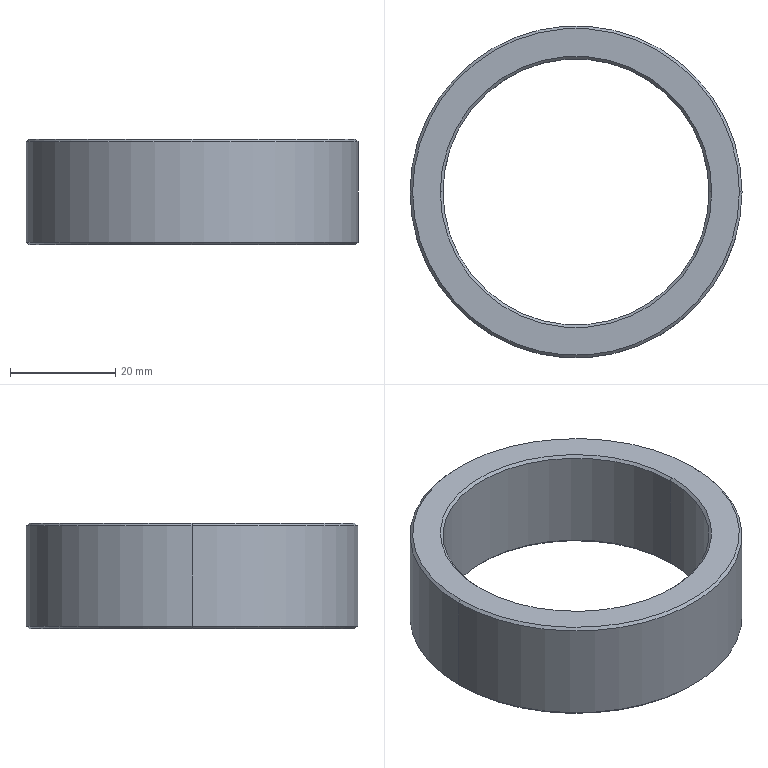Part | SolidWorks | features Chamfer 1, Extrusion 1 | 1 solid | 14 faces | box 63 x 63 x 20 mm | volume 22197 mm3 | cone 8 | cylinder 4 | plane 2 | commonest cylinder face diameters 50.5 x2 63 x2
STEP:
#1=CARTESIAN_POINT('',(31.,0.,20.));
#2=VERTEX_POINT('',#1);
#3=CARTESIAN_POINT('',(-31.,0.,20.));
#4=VERTEX_POINT('',#3);
#5=CARTESIAN_POINT('',(0.,0.,20.));
#6=DIRECTION('',(0.,0.,1.));
#7=DIRECTION('',(1.,0.,0.));
#8=AXIS2_PLACEMENT_3D('',#5,#6,#7);
#9=CIRCLE('',#8,31.);
#10=EDGE_CURVE('',#2,#4,#9,.T.);
#11=ORIENTED_EDGE('',*,*,#10,.F.);
#12=CARTESIAN_POINT('',(31.5,0.,19.5));
#13=VERTEX_POINT('',#12);
#14=CARTESIAN_POINT('',(31.,0.,20.));
#15=DIRECTION('',(0.7071,0.,-0.7071));
#16=VECTOR('',#15,1000.);
#17=LINE('',#14,#16);
#18=EDGE_CURVE('',#2,#13,#17,.T.);
#19=ORIENTED_EDGE('',*,*,#18,.T.);
#20=CARTESIAN_POINT('',(-31.5,0.,19.5));
#21=VERTEX_POINT('',#20);
#22=CARTESIAN_POINT('',(0.,0.,19.5));
#23=DIRECTION('',(0.,0.,-1.));
#24=DIRECTION('',(1.,0.,0.));
#25=AXIS2_PLACEMENT_3D('',#22,#23,#24);
#26=CIRCLE('',#25,31.5);
#27=EDGE_CURVE('',#21,#13,#26,.T.);
#28=ORIENTED_EDGE('',*,*,#27,.F.);
#29=CARTESIAN_POINT('',(-31.,0.,20.));
#30=DIRECTION('',(-0.7071,0.,-0.7071));
#31=VECTOR('',#30,1000.);
#32=LINE('',#29,#31);
#33=EDGE_CURVE('',#4,#21,#32,.T.);
#34=ORIENTED_EDGE('',*,*,#33,.F.);
#35=EDGE_LOOP('',(#11,#19,#28,#34));
#36=FACE_OUTER_BOUND('',#35,.T.);
#37=CARTESIAN_POINT('',(0.,0.,20.));
#38=DIRECTION('',(0.,0.,-1.));
#39=DIRECTION('',(-1.,0.,0.));
#40=AXIS2_PLACEMENT_3D('',#37,#38,#39);
#41=CONICAL_SURFACE('',#40,31.,0.7854);
#42=ADVANCED_FACE('',(#36),#41,.T.);
#43=CARTESIAN_POINT('',(-25.25,0.,19.5));
#44=VERTEX_POINT('',#43);
#45=CARTESIAN_POINT('',(25.25,0.,19.5));
#46=VERTEX_POINT('',#45);
#47=CARTESIAN_POINT('',(0.,0.,19.5));
#48=DIRECTION('',(0.,0.,1.));
#49=DIRECTION('',(1.,0.,0.));
#50=AXIS2_PLACEMENT_3D('',#47,#48,#49);
#51=CIRCLE('',#50,25.25);
#52=EDGE_CURVE('',#44,#46,#51,.T.);
#53=ORIENTED_EDGE('',*,*,#52,.F.);
#54=CARTESIAN_POINT('',(-25.75,0.,20.));
#55=VERTEX_POINT('',#54);
#56=CARTESIAN_POINT('',(-25.25,0.,19.5));
#57=DIRECTION('',(-0.7071,0.,0.7071));
#58=VECTOR('',#57,1000.);
#59=LINE('',#56,#58);
#60=EDGE_CURVE('',#44,#55,#59,.T.);
#61=ORIENTED_EDGE('',*,*,#60,.T.);
#62=CARTESIAN_POINT('',(25.75,0.,20.));
#63=VERTEX_POINT('',#62);
#64=CARTESIAN_POINT('',(0.,0.,20.));
#65=DIRECTION('',(0.,0.,-1.));
#66=DIRECTION('',(1.,0.,0.));
#67=AXIS2_PLACEMENT_3D('',#64,#65,#66);
#68=CIRCLE('',#67,25.75);
#69=EDGE_CURVE('',#63,#55,#68,.T.);
#70=ORIENTED_EDGE('',*,*,#69,.F.);
#71=CARTESIAN_POINT('',(25.25,0.,19.5));
#72=DIRECTION('',(0.7071,0.,0.7071));
#73=VECTOR('',#72,1000.);
#74=LINE('',#71,#73);
#75=EDGE_CURVE('',#46,#63,#74,.T.);
#76=ORIENTED_EDGE('',*,*,#75,.F.);
#77=EDGE_LOOP('',(#53,#61,#70,#76));
#78=FACE_OUTER_BOUND('',#77,.T.);
#79=CARTESIAN_POINT('',(0.,0.,19.5));
#80=DIRECTION('',(0.,0.,1.));
#81=DIRECTION('',(1.,0.,0.));
#82=AXIS2_PLACEMENT_3D('',#79,#80,#81);
#83=CONICAL_SURFACE('',#82,25.25,0.7854);
#84=ADVANCED_FACE('',(#78),#83,.F.);
#85=CARTESIAN_POINT('',(-31.,0.,0.));
#86=VERTEX_POINT('',#85);
#87=CARTESIAN_POINT('',(31.,0.,0.));
#88=VERTEX_POINT('',#87);
#89=CARTESIAN_POINT('',(0.,0.,0.));
#90=DIRECTION('',(0.,0.,-1.));
#91=DIRECTION('',(1.,0.,0.));
#92=AXIS2_PLACEMENT_3D('',#89,#90,#91);
#93=CIRCLE('',#92,31.);
#94=EDGE_CURVE('',#86,#88,#93,.T.);
#95=ORIENTED_EDGE('',*,*,#94,.F.);
#96=CARTESIAN_POINT('',(-31.5,0.,0.5));
#97=VERTEX_POINT('',#96);
#98=CARTESIAN_POINT('',(-31.5,0.,0.5));
#99=DIRECTION('',(-0.7071,0.,0.7071));
#100=VECTOR('',#99,1000.);
#101=LINE('',#98,#100);
#102=EDGE_CURVE('',#86,#97,#101,.T.);
#103=ORIENTED_EDGE('',*,*,#102,.T.);
#104=CARTESIAN_POINT('',(31.5,0.,0.5));
#105=VERTEX_POINT('',#104);
#106=CARTESIAN_POINT('',(0.,0.,0.5));
#107=DIRECTION('',(0.,0.,1.));
#108=DIRECTION('',(1.,0.,0.));
#109=AXIS2_PLACEMENT_3D('',#106,#107,#108);
#110=CIRCLE('',#109,31.5);
#111=EDGE_CURVE('',#105,#97,#110,.T.);
#112=ORIENTED_EDGE('',*,*,#111,.F.);
#113=CARTESIAN_POINT('',(31.5,0.,0.5));
#114=DIRECTION('',(0.7071,0.,0.7071));
#115=VECTOR('',#114,1000.);
#116=LINE('',#113,#115);
#117=EDGE_CURVE('',#88,#105,#116,.T.);
#118=ORIENTED_EDGE('',*,*,#117,.F.);
#119=EDGE_LOOP('',(#95,#103,#112,#118));
#120=FACE_OUTER_BOUND('',#119,.T.);
#121=CARTESIAN_POINT('',(0.,0.,0.5));
#122=DIRECTION('',(0.,0.,1.));
#123=DIRECTION('',(1.,0.,0.));
#124=AXIS2_PLACEMENT_3D('',#121,#122,#123);
#125=CONICAL_SURFACE('',#124,31.5,0.7854);
#126=ADVANCED_FACE('',(#120),#125,.T.);
#127=CARTESIAN_POINT('',(25.25,0.,0.5));
#128=VERTEX_POINT('',#127);
#129=CARTESIAN_POINT('',(-25.25,0.,0.5));
#130=VERTEX_POINT('',#129);
#131=CARTESIAN_POINT('',(0.,0.,0.5));
#132=DIRECTION('',(0.,0.,-1.));
#133=DIRECTION('',(1.,0.,0.));
#134=AXIS2_PLACEMENT_3D('',#131,#132,#133);
#135=CIRCLE('',#134,25.25);
#136=EDGE_CURVE('',#128,#130,#135,.T.);
#137=ORIENTED_EDGE('',*,*,#136,.F.);
#138=CARTESIAN_POINT('',(25.75,0.,0.));
#139=VERTEX_POINT('',#138);
#140=CARTESIAN_POINT('',(25.75,0.,0.));
#141=DIRECTION('',(0.7071,0.,-0.7071));
#142=VECTOR('',#141,1000.);
#143=LINE('',#140,#142);
#144=EDGE_CURVE('',#128,#139,#143,.T.);
#145=ORIENTED_EDGE('',*,*,#144,.T.);
#146=CARTESIAN_POINT('',(-25.75,0.,0.));
#147=VERTEX_POINT('',#146);
#148=CARTESIAN_POINT('',(0.,0.,0.));
#149=DIRECTION('',(0.,0.,1.));
#150=DIRECTION('',(1.,0.,0.));
#151=AXIS2_PLACEMENT_3D('',#148,#149,#150);
#152=CIRCLE('',#151,25.75);
#153=EDGE_CURVE('',#147,#139,#152,.T.);
#154=ORIENTED_EDGE('',*,*,#153,.F.);
#155=CARTESIAN_POINT('',(-25.75,0.,0.));
#156=DIRECTION('',(-0.7071,0.,-0.7071));
#157=VECTOR('',#156,1000.);
#158=LINE('',#155,#157);
#159=EDGE_CURVE('',#130,#147,#158,.T.);
#160=ORIENTED_EDGE('',*,*,#159,.F.);
#161=EDGE_LOOP('',(#137,#145,#154,#160));
#162=FACE_OUTER_BOUND('',#161,.T.);
#163=CARTESIAN_POINT('',(0.,0.,0.));
#164=DIRECTION('',(0.,0.,-1.));
#165=DIRECTION('',(-1.,0.,0.));
#166=AXIS2_PLACEMENT_3D('',#163,#164,#165);
#167=CONICAL_SURFACE('',#166,25.75,0.7854);
#168=ADVANCED_FACE('',(#162),#167,.F.);
#169=ORIENTED_EDGE('',*,*,#52,.T.);
#170=CARTESIAN_POINT('',(25.25,0.,20.));
#171=DIRECTION('',(0.,0.,-1.));
#172=VECTOR('',#171,1000.);
#173=LINE('',#170,#172);
#174=EDGE_CURVE('',#46,#128,#173,.T.);
#175=ORIENTED_EDGE('',*,*,#174,.T.);
#176=ORIENTED_EDGE('',*,*,#136,.T.);
#177=CARTESIAN_POINT('',(-25.25,0.,20.));
#178=DIRECTION('',(0.,0.,-1.));
#179=VECTOR('',#178,1000.);
#180=LINE('',#177,#179);
#181=EDGE_CURVE('',#44,#130,#180,.T.);
#182=ORIENTED_EDGE('',*,*,#181,.F.);
#183=EDGE_LOOP('',(#169,#175,#176,#182));
#184=FACE_OUTER_BOUND('',#183,.T.);
#185=CARTESIAN_POINT('',(0.,0.,20.));
#186=DIRECTION('',(0.,0.,-1.));
#187=DIRECTION('',(-1.,0.,0.));
#188=AXIS2_PLACEMENT_3D('',#185,#186,#187);
#189=CYLINDRICAL_SURFACE('',#188,25.25);
#190=ADVANCED_FACE('',(#184),#189,.F.);
#191=ORIENTED_EDGE('',*,*,#27,.T.);
#192=CARTESIAN_POINT('',(31.5,0.,20.));
#193=DIRECTION('',(0.,0.,-1.));
#194=VECTOR('',#193,1000.);
#195=LINE('',#192,#194);
#196=EDGE_CURVE('',#13,#105,#195,.T.);
#197=ORIENTED_EDGE('',*,*,#196,.T.);
#198=ORIENTED_EDGE('',*,*,#111,.T.);
#199=CARTESIAN_POINT('',(-31.5,0.,20.));
#200=DIRECTION('',(0.,0.,-1.));
#201=VECTOR('',#200,1000.);
#202=LINE('',#199,#201);
#203=EDGE_CURVE('',#21,#97,#202,.T.);
#204=ORIENTED_EDGE('',*,*,#203,.F.);
#205=EDGE_LOOP('',(#191,#197,#198,#204));
#206=FACE_OUTER_BOUND('',#205,.T.);
#207=CARTESIAN_POINT('',(0.,0.,20.));
#208=DIRECTION('',(0.,0.,-1.));
#209=DIRECTION('',(-1.,0.,0.));
#210=AXIS2_PLACEMENT_3D('',#207,#208,#209);
#211=CYLINDRICAL_SURFACE('',#210,31.5);
#212=ADVANCED_FACE('',(#206),#211,.T.);
#213=ORIENTED_EDGE('',*,*,#69,.T.);
#214=CARTESIAN_POINT('',(0.,0.,20.));
#215=DIRECTION('',(0.,0.,-1.));
#216=DIRECTION('',(1.,0.,0.));
#217=AXIS2_PLACEMENT_3D('',#214,#215,#216);
#218=CIRCLE('',#217,25.75);
#219=EDGE_CURVE('',#55,#63,#218,.T.);
#220=ORIENTED_EDGE('',*,*,#219,.T.);
#221=EDGE_LOOP('',(#213,#220));
#222=FACE_BOUND('',#221,.T.);
#223=CARTESIAN_POINT('',(0.,0.,20.));
#224=DIRECTION('',(0.,0.,1.));
#225=DIRECTION('',(1.,0.,0.));
#226=AXIS2_PLACEMENT_3D('',#223,#224,#225);
#227=CIRCLE('',#226,31.);
#228=EDGE_CURVE('',#4,#2,#227,.T.);
#229=ORIENTED_EDGE('',*,*,#228,.T.);
#230=ORIENTED_EDGE('',*,*,#10,.T.);
#231=EDGE_LOOP('',(#229,#230));
#232=FACE_OUTER_BOUND('',#231,.T.);
#233=CARTESIAN_POINT('',(0.,0.,20.));
#234=DIRECTION('',(0.,0.,1.));
#235=DIRECTION('',(1.,0.,0.));
#236=AXIS2_PLACEMENT_3D('',#233,#234,#235);
#237=PLANE('',#236);
#238=ADVANCED_FACE('',(#222,#232),#237,.T.);
#239=ORIENTED_EDGE('',*,*,#153,.T.);
#240=CARTESIAN_POINT('',(0.,0.,0.));
#241=DIRECTION('',(0.,0.,1.));
#242=DIRECTION('',(1.,0.,0.));
#243=AXIS2_PLACEMENT_3D('',#240,#241,#242);
#244=CIRCLE('',#243,25.75);
#245=EDGE_CURVE('',#139,#147,#244,.T.);
#246=ORIENTED_EDGE('',*,*,#245,.T.);
#247=EDGE_LOOP('',(#239,#246));
#248=FACE_BOUND('',#247,.T.);
#249=CARTESIAN_POINT('',(0.,0.,0.));
#250=DIRECTION('',(0.,0.,-1.));
#251=DIRECTION('',(1.,0.,0.));
#252=AXIS2_PLACEMENT_3D('',#249,#250,#251);
#253=CIRCLE('',#252,31.);
#254=EDGE_CURVE('',#88,#86,#253,.T.);
#255=ORIENTED_EDGE('',*,*,#254,.T.);
#256=ORIENTED_EDGE('',*,*,#94,.T.);
#257=EDGE_LOOP('',(#255,#256));
#258=FACE_OUTER_BOUND('',#257,.T.);
#259=CARTESIAN_POINT('',(0.,0.,0.));
#260=DIRECTION('',(0.,0.,1.));
#261=DIRECTION('',(1.,0.,0.));
#262=AXIS2_PLACEMENT_3D('',#259,#260,#261);
#263=PLANE('',#262);
#264=ADVANCED_FACE('',(#248,#258),#263,.F.);
#265=ORIENTED_EDGE('',*,*,#196,.F.);
#266=CARTESIAN_POINT('',(0.,0.,19.5));
#267=DIRECTION('',(0.,0.,-1.));
#268=DIRECTION('',(1.,0.,0.));
#269=AXIS2_PLACEMENT_3D('',#266,#267,#268);
#270=CIRCLE('',#269,31.5);
#271=EDGE_CURVE('',#13,#21,#270,.T.);
#272=ORIENTED_EDGE('',*,*,#271,.T.);
#273=ORIENTED_EDGE('',*,*,#203,.T.);
#274=CARTESIAN_POINT('',(0.,0.,0.5));
#275=DIRECTION('',(0.,0.,1.));
#276=DIRECTION('',(1.,0.,0.));
#277=AXIS2_PLACEMENT_3D('',#274,#275,#276);
#278=CIRCLE('',#277,31.5);
#279=EDGE_CURVE('',#97,#105,#278,.T.);
#280=ORIENTED_EDGE('',*,*,#279,.T.);
#281=EDGE_LOOP('',(#265,#272,#273,#280));
#282=FACE_OUTER_BOUND('',#281,.T.);
#283=CARTESIAN_POINT('',(0.,0.,20.));
#284=DIRECTION('',(0.,0.,-1.));
#285=DIRECTION('',(-1.,0.,0.));
#286=AXIS2_PLACEMENT_3D('',#283,#284,#285);
#287=CYLINDRICAL_SURFACE('',#286,31.5);
#288=ADVANCED_FACE('',(#282),#287,.T.);
#289=ORIENTED_EDGE('',*,*,#174,.F.);
#290=CARTESIAN_POINT('',(0.,0.,19.5));
#291=DIRECTION('',(0.,0.,1.));
#292=DIRECTION('',(1.,0.,0.));
#293=AXIS2_PLACEMENT_3D('',#290,#291,#292);
#294=CIRCLE('',#293,25.25);
#295=EDGE_CURVE('',#46,#44,#294,.T.);
#296=ORIENTED_EDGE('',*,*,#295,.T.);
#297=ORIENTED_EDGE('',*,*,#181,.T.);
#298=CARTESIAN_POINT('',(0.,0.,0.5));
#299=DIRECTION('',(0.,0.,-1.));
#300=DIRECTION('',(1.,0.,0.));
#301=AXIS2_PLACEMENT_3D('',#298,#299,#300);
#302=CIRCLE('',#301,25.25);
#303=EDGE_CURVE('',#130,#128,#302,.T.);
#304=ORIENTED_EDGE('',*,*,#303,.T.);
#305=EDGE_LOOP('',(#289,#296,#297,#304));
#306=FACE_OUTER_BOUND('',#305,.T.);
#307=CARTESIAN_POINT('',(0.,0.,20.));
#308=DIRECTION('',(0.,0.,-1.));
#309=DIRECTION('',(-1.,0.,0.));
#310=AXIS2_PLACEMENT_3D('',#307,#308,#309);
#311=CYLINDRICAL_SURFACE('',#310,25.25);
#312=ADVANCED_FACE('',(#306),#311,.F.);
#313=ORIENTED_EDGE('',*,*,#144,.F.);
#314=ORIENTED_EDGE('',*,*,#303,.F.);
#315=ORIENTED_EDGE('',*,*,#159,.T.);
#316=ORIENTED_EDGE('',*,*,#245,.F.);
#317=EDGE_LOOP('',(#313,#314,#315,#316));
#318=FACE_OUTER_BOUND('',#317,.T.);
#319=CARTESIAN_POINT('',(0.,0.,0.));
#320=DIRECTION('',(0.,0.,-1.));
#321=DIRECTION('',(-1.,0.,0.));
#322=AXIS2_PLACEMENT_3D('',#319,#320,#321);
#323=CONICAL_SURFACE('',#322,25.75,0.7854);
#324=ADVANCED_FACE('',(#318),#323,.F.);
#325=ORIENTED_EDGE('',*,*,#102,.F.);
#326=ORIENTED_EDGE('',*,*,#254,.F.);
#327=ORIENTED_EDGE('',*,*,#117,.T.);
#328=ORIENTED_EDGE('',*,*,#279,.F.);
#329=EDGE_LOOP('',(#325,#326,#327,#328));
#330=FACE_OUTER_BOUND('',#329,.T.);
#331=CARTESIAN_POINT('',(0.,0.,0.5));
#332=DIRECTION('',(0.,0.,1.));
#333=DIRECTION('',(1.,0.,0.));
#334=AXIS2_PLACEMENT_3D('',#331,#332,#333);
#335=CONICAL_SURFACE('',#334,31.5,0.7854);
#336=ADVANCED_FACE('',(#330),#335,.T.);
#337=ORIENTED_EDGE('',*,*,#60,.F.);
#338=ORIENTED_EDGE('',*,*,#295,.F.);
#339=ORIENTED_EDGE('',*,*,#75,.T.);
#340=ORIENTED_EDGE('',*,*,#219,.F.);
#341=EDGE_LOOP('',(#337,#338,#339,#340));
#342=FACE_OUTER_BOUND('',#341,.T.);
#343=CARTESIAN_POINT('',(0.,0.,19.5));
#344=DIRECTION('',(0.,0.,1.));
#345=DIRECTION('',(1.,0.,0.));
#346=AXIS2_PLACEMENT_3D('',#343,#344,#345);
#347=CONICAL_SURFACE('',#346,25.25,0.7854);
#348=ADVANCED_FACE('',(#342),#347,.F.);
#349=ORIENTED_EDGE('',*,*,#18,.F.);
#350=ORIENTED_EDGE('',*,*,#228,.F.);
#351=ORIENTED_EDGE('',*,*,#33,.T.);
#352=ORIENTED_EDGE('',*,*,#271,.F.);
#353=EDGE_LOOP('',(#349,#350,#351,#352));
#354=FACE_OUTER_BOUND('',#353,.T.);
#355=CARTESIAN_POINT('',(0.,0.,20.));
#356=DIRECTION('',(0.,0.,-1.));
#357=DIRECTION('',(-1.,0.,0.));
#358=AXIS2_PLACEMENT_3D('',#355,#356,#357);
#359=CONICAL_SURFACE('',#358,31.,0.7854);
#360=ADVANCED_FACE('',(#354),#359,.T.);
#361=CLOSED_SHELL('',(#42,#84,#126,#168,#190,#212,#238,#264,#288,#312,#324,#336,#348,#360));
#362=MANIFOLD_SOLID_BREP('',#361);
#363=CARTESIAN_POINT('',(0.,0.,0.));
#364=DIRECTION('',(0.,0.,1.));
#365=DIRECTION('',(1.,0.,0.));
#366=AXIS2_PLACEMENT_3D('',#363,#364,#365);
#367=(LENGTH_UNIT()NAMED_UNIT(*)SI_UNIT(.MILLI.,.METRE.));
#368=UNCERTAINTY_MEASURE_WITH_UNIT(LENGTH_MEASURE(0.00001),#367,'','');
#369=(NAMED_UNIT(*)PLANE_ANGLE_UNIT()SI_UNIT($,.RADIAN.));
#370=(NAMED_UNIT(*)SI_UNIT($,.STERADIAN.)SOLID_ANGLE_UNIT());
#371=(GEOMETRIC_REPRESENTATION_CONTEXT(3)GLOBAL_UNCERTAINTY_ASSIGNED_CONTEXT((#368))GLOBAL_UNIT_ASSIGNED_CONTEXT((#367,#369,#370))REPRESENTATION_CONTEXT('',''));
#372=ADVANCED_BREP_SHAPE_REPRESENTATION('',(#362,#366),#371);